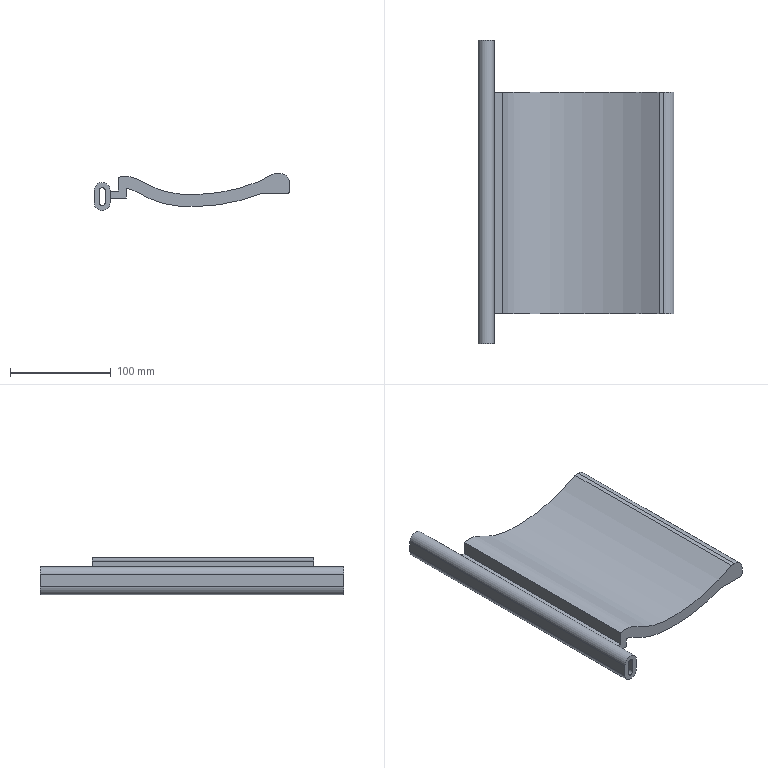Part | SolidWorks | features ExtruThin 1, ICE 1 | 1 solid | 25 faces | box 194.613 x 302 x 37.008 mm | volume 615517 mm3 | plane 15 | cylinder 8 | spline 2 | commonest cylinder face diameters 6 x4 16 x3 20 x1
STEP:
#1=CARTESIAN_POINT('',(3.,2.,-11.497));
#2=VERTEX_POINT('',#1);
#3=CARTESIAN_POINT('',(0.,2.,-14.497));
#4=VERTEX_POINT('',#3);
#5=CARTESIAN_POINT('',(0.,2.,-11.497));
#6=DIRECTION('',(0.,1.,0.));
#7=DIRECTION('',(0.,0.,1.));
#8=AXIS2_PLACEMENT_3D('',#5,#6,#7);
#9=CIRCLE('',#8,3.);
#10=EDGE_CURVE('',#2,#4,#9,.T.);
#11=ORIENTED_EDGE('',*,*,#10,.T.);
#12=CARTESIAN_POINT('',(0.,-300.,-14.497));
#13=VERTEX_POINT('',#12);
#14=CARTESIAN_POINT('',(0.,2.,-14.497));
#15=DIRECTION('',(0.,-1.,0.));
#16=VECTOR('',#15,1000.);
#17=LINE('',#14,#16);
#18=EDGE_CURVE('',#4,#13,#17,.T.);
#19=ORIENTED_EDGE('',*,*,#18,.T.);
#20=CARTESIAN_POINT('',(3.,-300.,-11.497));
#21=VERTEX_POINT('',#20);
#22=CARTESIAN_POINT('',(0.,-300.,-11.497));
#23=DIRECTION('',(0.,1.,0.));
#24=DIRECTION('',(0.,0.,1.));
#25=AXIS2_PLACEMENT_3D('',#22,#23,#24);
#26=CIRCLE('',#25,3.);
#27=EDGE_CURVE('',#21,#13,#26,.T.);
#28=ORIENTED_EDGE('',*,*,#27,.F.);
#29=CARTESIAN_POINT('',(3.,2.,-11.497));
#30=DIRECTION('',(0.,-1.,0.));
#31=VECTOR('',#30,1000.);
#32=LINE('',#29,#31);
#33=EDGE_CURVE('',#2,#21,#32,.T.);
#34=ORIENTED_EDGE('',*,*,#33,.F.);
#35=EDGE_LOOP('',(#11,#19,#28,#34));
#36=FACE_OUTER_BOUND('',#35,.T.);
#37=CARTESIAN_POINT('',(0.,2.,-11.497));
#38=DIRECTION('',(0.,-1.,0.));
#39=DIRECTION('',(0.,0.,-1.));
#40=AXIS2_PLACEMENT_3D('',#37,#38,#39);
#41=CYLINDRICAL_SURFACE('',#40,3.);
#42=ADVANCED_FACE('',(#36),#41,.F.);
#43=CARTESIAN_POINT('',(0.,2.,-19.497));
#44=VERTEX_POINT('',#43);
#45=CARTESIAN_POINT('',(-8.,2.,-11.497));
#46=VERTEX_POINT('',#45);
#47=CARTESIAN_POINT('',(0.,2.,-11.497));
#48=DIRECTION('',(0.,1.,0.));
#49=DIRECTION('',(1.,0.,0.));
#50=AXIS2_PLACEMENT_3D('',#47,#48,#49);
#51=CIRCLE('',#50,8.);
#52=EDGE_CURVE('',#44,#46,#51,.T.);
#53=ORIENTED_EDGE('',*,*,#52,.F.);
#54=CARTESIAN_POINT('',(0.,-300.,-19.497));
#55=VERTEX_POINT('',#54);
#56=CARTESIAN_POINT('',(0.,2.,-19.497));
#57=DIRECTION('',(0.,-1.,0.));
#58=VECTOR('',#57,1000.);
#59=LINE('',#56,#58);
#60=EDGE_CURVE('',#44,#55,#59,.T.);
#61=ORIENTED_EDGE('',*,*,#60,.T.);
#62=CARTESIAN_POINT('',(-8.,-300.,-11.497));
#63=VERTEX_POINT('',#62);
#64=CARTESIAN_POINT('',(0.,-300.,-11.497));
#65=DIRECTION('',(0.,1.,0.));
#66=DIRECTION('',(1.,0.,0.));
#67=AXIS2_PLACEMENT_3D('',#64,#65,#66);
#68=CIRCLE('',#67,8.);
#69=EDGE_CURVE('',#55,#63,#68,.T.);
#70=ORIENTED_EDGE('',*,*,#69,.T.);
#71=CARTESIAN_POINT('',(-8.,2.,-11.497));
#72=DIRECTION('',(0.,-1.,0.));
#73=VECTOR('',#72,1000.);
#74=LINE('',#71,#73);
#75=EDGE_CURVE('',#46,#63,#74,.T.);
#76=ORIENTED_EDGE('',*,*,#75,.F.);
#77=EDGE_LOOP('',(#53,#61,#70,#76));
#78=FACE_OUTER_BOUND('',#77,.T.);
#79=CARTESIAN_POINT('',(0.,2.,-11.497));
#80=DIRECTION('',(0.,-1.,0.));
#81=DIRECTION('',(0.,0.,-1.));
#82=AXIS2_PLACEMENT_3D('',#79,#80,#81);
#83=CYLINDRICAL_SURFACE('',#82,8.);
#84=ADVANCED_FACE('',(#78),#83,.T.);
#85=CARTESIAN_POINT('',(8.,2.,-11.497));
#86=VERTEX_POINT('',#85);
#87=CARTESIAN_POINT('',(0.,2.,-11.497));
#88=DIRECTION('',(0.,1.,0.));
#89=DIRECTION('',(1.,0.,0.));
#90=AXIS2_PLACEMENT_3D('',#87,#88,#89);
#91=CIRCLE('',#90,8.);
#92=EDGE_CURVE('',#86,#44,#91,.T.);
#93=ORIENTED_EDGE('',*,*,#92,.T.);
#94=ORIENTED_EDGE('',*,*,#52,.T.);
#95=CARTESIAN_POINT('',(-8.,2.,0.5032));
#96=VERTEX_POINT('',#95);
#97=CARTESIAN_POINT('',(-8.,2.,-11.497));
#98=DIRECTION('',(0.,0.,1.));
#99=VECTOR('',#98,1000.);
#100=LINE('',#97,#99);
#101=EDGE_CURVE('',#46,#96,#100,.T.);
#102=ORIENTED_EDGE('',*,*,#101,.T.);
#103=CARTESIAN_POINT('',(8.,2.,0.5032));
#104=VERTEX_POINT('',#103);
#105=CARTESIAN_POINT('',(0.,2.,0.5032));
#106=DIRECTION('',(0.,1.,0.));
#107=DIRECTION('',(1.,0.,0.));
#108=AXIS2_PLACEMENT_3D('',#105,#106,#107);
#109=CIRCLE('',#108,8.);
#110=EDGE_CURVE('',#96,#104,#109,.T.);
#111=ORIENTED_EDGE('',*,*,#110,.T.);
#112=CARTESIAN_POINT('',(8.,2.,-11.497));
#113=DIRECTION('',(0.,0.,-1.));
#114=VECTOR('',#113,1000.);
#115=LINE('',#112,#114);
#116=EDGE_CURVE('',#104,#86,#115,.T.);
#117=ORIENTED_EDGE('',*,*,#116,.T.);
#118=EDGE_LOOP('',(#93,#94,#102,#111,#117));
#119=FACE_OUTER_BOUND('',#118,.T.);
#120=CARTESIAN_POINT('',(-3.,2.,-11.497));
#121=VERTEX_POINT('',#120);
#122=CARTESIAN_POINT('',(-3.,2.,0.5032));
#123=VERTEX_POINT('',#122);
#124=CARTESIAN_POINT('',(-3.,2.,-11.497));
#125=DIRECTION('',(0.,0.,1.));
#126=VECTOR('',#125,1000.);
#127=LINE('',#124,#126);
#128=EDGE_CURVE('',#121,#123,#127,.T.);
#129=ORIENTED_EDGE('',*,*,#128,.F.);
#130=CARTESIAN_POINT('',(0.,2.,-11.497));
#131=DIRECTION('',(0.,1.,0.));
#132=DIRECTION('',(0.,0.,1.));
#133=AXIS2_PLACEMENT_3D('',#130,#131,#132);
#134=CIRCLE('',#133,3.);
#135=EDGE_CURVE('',#4,#121,#134,.T.);
#136=ORIENTED_EDGE('',*,*,#135,.F.);
#137=ORIENTED_EDGE('',*,*,#10,.F.);
#138=CARTESIAN_POINT('',(3.,2.,0.5032));
#139=VERTEX_POINT('',#138);
#140=CARTESIAN_POINT('',(3.,2.,-11.497));
#141=DIRECTION('',(0.,0.,-1.));
#142=VECTOR('',#141,1000.);
#143=LINE('',#140,#142);
#144=EDGE_CURVE('',#139,#2,#143,.T.);
#145=ORIENTED_EDGE('',*,*,#144,.F.);
#146=CARTESIAN_POINT('',(0.,2.,0.5032));
#147=DIRECTION('',(0.,1.,0.));
#148=DIRECTION('',(0.,0.,1.));
#149=AXIS2_PLACEMENT_3D('',#146,#147,#148);
#150=CIRCLE('',#149,3.);
#151=EDGE_CURVE('',#123,#139,#150,.T.);
#152=ORIENTED_EDGE('',*,*,#151,.F.);
#153=EDGE_LOOP('',(#129,#136,#137,#145,#152));
#154=FACE_BOUND('',#153,.T.);
#155=CARTESIAN_POINT('',(0.,2.,-11.497));
#156=DIRECTION('',(0.,1.,0.));
#157=DIRECTION('',(0.,0.,1.));
#158=AXIS2_PLACEMENT_3D('',#155,#156,#157);
#159=PLANE('',#158);
#160=ADVANCED_FACE('',(#119,#154),#159,.T.);
#161=ORIENTED_EDGE('',*,*,#60,.F.);
#162=ORIENTED_EDGE('',*,*,#92,.F.);
#163=CARTESIAN_POINT('',(8.,-300.,-11.497));
#164=VERTEX_POINT('',#163);
#165=CARTESIAN_POINT('',(8.,2.,-11.497));
#166=DIRECTION('',(0.,-1.,0.));
#167=VECTOR('',#166,1000.);
#168=LINE('',#165,#167);
#169=EDGE_CURVE('',#86,#164,#168,.T.);
#170=ORIENTED_EDGE('',*,*,#169,.T.);
#171=CARTESIAN_POINT('',(0.,-300.,-11.497));
#172=DIRECTION('',(0.,1.,0.));
#173=DIRECTION('',(1.,0.,0.));
#174=AXIS2_PLACEMENT_3D('',#171,#172,#173);
#175=CIRCLE('',#174,8.);
#176=EDGE_CURVE('',#164,#55,#175,.T.);
#177=ORIENTED_EDGE('',*,*,#176,.T.);
#178=EDGE_LOOP('',(#161,#162,#170,#177));
#179=FACE_OUTER_BOUND('',#178,.T.);
#180=CARTESIAN_POINT('',(0.,2.,-11.497));
#181=DIRECTION('',(0.,-1.,0.));
#182=DIRECTION('',(0.,0.,-1.));
#183=AXIS2_PLACEMENT_3D('',#180,#181,#182);
#184=CYLINDRICAL_SURFACE('',#183,8.);
#185=ADVANCED_FACE('',(#179),#184,.T.);
#186=ORIENTED_EDGE('',*,*,#75,.T.);
#187=CARTESIAN_POINT('',(-8.,-300.,0.5032));
#188=VERTEX_POINT('',#187);
#189=CARTESIAN_POINT('',(-8.,-300.,-11.497));
#190=DIRECTION('',(0.,0.,1.));
#191=VECTOR('',#190,1000.);
#192=LINE('',#189,#191);
#193=EDGE_CURVE('',#63,#188,#192,.T.);
#194=ORIENTED_EDGE('',*,*,#193,.T.);
#195=CARTESIAN_POINT('',(-8.,2.,0.5032));
#196=DIRECTION('',(0.,-1.,0.));
#197=VECTOR('',#196,1000.);
#198=LINE('',#195,#197);
#199=EDGE_CURVE('',#96,#188,#198,.T.);
#200=ORIENTED_EDGE('',*,*,#199,.F.);
#201=ORIENTED_EDGE('',*,*,#101,.F.);
#202=EDGE_LOOP('',(#186,#194,#200,#201));
#203=FACE_OUTER_BOUND('',#202,.T.);
#204=CARTESIAN_POINT('',(-8.,2.,-11.497));
#205=DIRECTION('',(1.,0.,0.));
#206=DIRECTION('',(0.,0.,-1.));
#207=AXIS2_PLACEMENT_3D('',#204,#205,#206);
#208=PLANE('',#207);
#209=ADVANCED_FACE('',(#203),#208,.F.);
#210=ORIENTED_EDGE('',*,*,#199,.T.);
#211=CARTESIAN_POINT('',(8.,-300.,0.5032));
#212=VERTEX_POINT('',#211);
#213=CARTESIAN_POINT('',(0.,-300.,0.5032));
#214=DIRECTION('',(0.,1.,0.));
#215=DIRECTION('',(1.,0.,0.));
#216=AXIS2_PLACEMENT_3D('',#213,#214,#215);
#217=CIRCLE('',#216,8.);
#218=EDGE_CURVE('',#188,#212,#217,.T.);
#219=ORIENTED_EDGE('',*,*,#218,.T.);
#220=CARTESIAN_POINT('',(8.,2.,0.5032));
#221=DIRECTION('',(0.,-1.,0.));
#222=VECTOR('',#221,1000.);
#223=LINE('',#220,#222);
#224=EDGE_CURVE('',#104,#212,#223,.T.);
#225=ORIENTED_EDGE('',*,*,#224,.F.);
#226=ORIENTED_EDGE('',*,*,#110,.F.);
#227=EDGE_LOOP('',(#210,#219,#225,#226));
#228=FACE_OUTER_BOUND('',#227,.T.);
#229=CARTESIAN_POINT('',(0.,2.,0.5032));
#230=DIRECTION('',(0.,-1.,0.));
#231=DIRECTION('',(0.,0.,-1.));
#232=AXIS2_PLACEMENT_3D('',#229,#230,#231);
#233=CYLINDRICAL_SURFACE('',#232,8.);
#234=ADVANCED_FACE('',(#228),#233,.T.);
#235=CARTESIAN_POINT('',(8.,-270.,-7.));
#236=VERTEX_POINT('',#235);
#237=CARTESIAN_POINT('',(8.,-50.,-7.));
#238=VERTEX_POINT('',#237);
#239=CARTESIAN_POINT('',(8.,-270.,-7.));
#240=DIRECTION('',(0.,1.,0.));
#241=VECTOR('',#240,1000.);
#242=LINE('',#239,#241);
#243=EDGE_CURVE('',#236,#238,#242,.T.);
#244=ORIENTED_EDGE('',*,*,#243,.F.);
#245=CARTESIAN_POINT('',(8.,-270.,0.));
#246=VERTEX_POINT('',#245);
#247=CARTESIAN_POINT('',(8.,-270.,0.));
#248=DIRECTION('',(0.,0.,1.));
#249=VECTOR('',#248,1000.);
#250=LINE('',#247,#249);
#251=EDGE_CURVE('',#236,#246,#250,.T.);
#252=ORIENTED_EDGE('',*,*,#251,.T.);
#253=CARTESIAN_POINT('',(8.,-50.,0.));
#254=VERTEX_POINT('',#253);
#255=CARTESIAN_POINT('',(8.,-270.,0.));
#256=DIRECTION('',(0.,1.,0.));
#257=VECTOR('',#256,1000.);
#258=LINE('',#255,#257);
#259=EDGE_CURVE('',#246,#254,#258,.T.);
#260=ORIENTED_EDGE('',*,*,#259,.T.);
#261=CARTESIAN_POINT('',(8.,-50.,0.));
#262=DIRECTION('',(0.,0.,1.));
#263=VECTOR('',#262,1000.);
#264=LINE('',#261,#263);
#265=EDGE_CURVE('',#238,#254,#264,.T.);
#266=ORIENTED_EDGE('',*,*,#265,.F.);
#267=EDGE_LOOP('',(#244,#252,#260,#266));
#268=FACE_BOUND('',#267,.T.);
#269=ORIENTED_EDGE('',*,*,#224,.T.);
#270=CARTESIAN_POINT('',(8.,-300.,-11.497));
#271=DIRECTION('',(0.,0.,-1.));
#272=VECTOR('',#271,1000.);
#273=LINE('',#270,#272);
#274=EDGE_CURVE('',#212,#164,#273,.T.);
#275=ORIENTED_EDGE('',*,*,#274,.T.);
#276=ORIENTED_EDGE('',*,*,#169,.F.);
#277=ORIENTED_EDGE('',*,*,#116,.F.);
#278=EDGE_LOOP('',(#269,#275,#276,#277));
#279=FACE_OUTER_BOUND('',#278,.T.);
#280=CARTESIAN_POINT('',(8.,2.,-11.497));
#281=DIRECTION('',(-1.,0.,0.));
#282=DIRECTION('',(0.,0.,1.));
#283=AXIS2_PLACEMENT_3D('',#280,#281,#282);
#284=PLANE('',#283);
#285=ADVANCED_FACE('',(#268,#279),#284,.F.);
#286=ORIENTED_EDGE('',*,*,#18,.F.);
#287=ORIENTED_EDGE('',*,*,#135,.T.);
#288=CARTESIAN_POINT('',(-3.,-300.,-11.497));
#289=VERTEX_POINT('',#288);
#290=CARTESIAN_POINT('',(-3.,2.,-11.497));
#291=DIRECTION('',(0.,-1.,0.));
#292=VECTOR('',#291,1000.);
#293=LINE('',#290,#292);
#294=EDGE_CURVE('',#121,#289,#293,.T.);
#295=ORIENTED_EDGE('',*,*,#294,.T.);
#296=CARTESIAN_POINT('',(0.,-300.,-11.497));
#297=DIRECTION('',(0.,1.,0.));
#298=DIRECTION('',(0.,0.,1.));
#299=AXIS2_PLACEMENT_3D('',#296,#297,#298);
#300=CIRCLE('',#299,3.);
#301=EDGE_CURVE('',#13,#289,#300,.T.);
#302=ORIENTED_EDGE('',*,*,#301,.F.);
#303=EDGE_LOOP('',(#286,#287,#295,#302));
#304=FACE_OUTER_BOUND('',#303,.T.);
#305=CARTESIAN_POINT('',(0.,2.,-11.497));
#306=DIRECTION('',(0.,-1.,0.));
#307=DIRECTION('',(0.,0.,-1.));
#308=AXIS2_PLACEMENT_3D('',#305,#306,#307);
#309=CYLINDRICAL_SURFACE('',#308,3.);
#310=ADVANCED_FACE('',(#304),#309,.F.);
#311=CARTESIAN_POINT('',(-3.,-300.,0.5032));
#312=VERTEX_POINT('',#311);
#313=CARTESIAN_POINT('',(-3.,2.,0.5032));
#314=DIRECTION('',(0.,-1.,0.));
#315=VECTOR('',#314,1000.);
#316=LINE('',#313,#315);
#317=EDGE_CURVE('',#123,#312,#316,.T.);
#318=ORIENTED_EDGE('',*,*,#317,.T.);
#319=CARTESIAN_POINT('',(-3.,-300.,-11.497));
#320=DIRECTION('',(0.,0.,1.));
#321=VECTOR('',#320,1000.);
#322=LINE('',#319,#321);
#323=EDGE_CURVE('',#289,#312,#322,.T.);
#324=ORIENTED_EDGE('',*,*,#323,.F.);
#325=ORIENTED_EDGE('',*,*,#294,.F.);
#326=ORIENTED_EDGE('',*,*,#128,.T.);
#327=EDGE_LOOP('',(#318,#324,#325,#326));
#328=FACE_OUTER_BOUND('',#327,.T.);
#329=CARTESIAN_POINT('',(-3.,2.,-11.497));
#330=DIRECTION('',(1.,0.,0.));
#331=DIRECTION('',(0.,0.,-1.));
#332=AXIS2_PLACEMENT_3D('',#329,#330,#331);
#333=PLANE('',#332);
#334=ADVANCED_FACE('',(#328),#333,.T.);
#335=CARTESIAN_POINT('',(3.,-300.,0.5032));
#336=VERTEX_POINT('',#335);
#337=CARTESIAN_POINT('',(3.,2.,0.5032));
#338=DIRECTION('',(0.,-1.,0.));
#339=VECTOR('',#338,1000.);
#340=LINE('',#337,#339);
#341=EDGE_CURVE('',#139,#336,#340,.T.);
#342=ORIENTED_EDGE('',*,*,#341,.T.);
#343=CARTESIAN_POINT('',(0.,-300.,0.5032));
#344=DIRECTION('',(0.,1.,0.));
#345=DIRECTION('',(0.,0.,1.));
#346=AXIS2_PLACEMENT_3D('',#343,#344,#345);
#347=CIRCLE('',#346,3.);
#348=EDGE_CURVE('',#312,#336,#347,.T.);
#349=ORIENTED_EDGE('',*,*,#348,.F.);
#350=ORIENTED_EDGE('',*,*,#317,.F.);
#351=ORIENTED_EDGE('',*,*,#151,.T.);
#352=EDGE_LOOP('',(#342,#349,#350,#351));
#353=FACE_OUTER_BOUND('',#352,.T.);
#354=CARTESIAN_POINT('',(0.,2.,0.5032));
#355=DIRECTION('',(0.,-1.,0.));
#356=DIRECTION('',(0.,0.,-1.));
#357=AXIS2_PLACEMENT_3D('',#354,#355,#356);
#358=CYLINDRICAL_SURFACE('',#357,3.);
#359=ADVANCED_FACE('',(#353),#358,.F.);
#360=ORIENTED_EDGE('',*,*,#33,.T.);
#361=CARTESIAN_POINT('',(3.,-300.,-11.497));
#362=DIRECTION('',(0.,0.,-1.));
#363=VECTOR('',#362,1000.);
#364=LINE('',#361,#363);
#365=EDGE_CURVE('',#336,#21,#364,.T.);
#366=ORIENTED_EDGE('',*,*,#365,.F.);
#367=ORIENTED_EDGE('',*,*,#341,.F.);
#368=ORIENTED_EDGE('',*,*,#144,.T.);
#369=EDGE_LOOP('',(#360,#366,#367,#368));
#370=FACE_OUTER_BOUND('',#369,.T.);
#371=CARTESIAN_POINT('',(3.,2.,-11.497));
#372=DIRECTION('',(-1.,0.,0.));
#373=DIRECTION('',(0.,0.,1.));
#374=AXIS2_PLACEMENT_3D('',#371,#372,#373);
#375=PLANE('',#374);
#376=ADVANCED_FACE('',(#370),#375,.T.);
#377=ORIENTED_EDGE('',*,*,#365,.T.);
#378=ORIENTED_EDGE('',*,*,#27,.T.);
#379=ORIENTED_EDGE('',*,*,#301,.T.);
#380=ORIENTED_EDGE('',*,*,#323,.T.);
#381=ORIENTED_EDGE('',*,*,#348,.T.);
#382=EDGE_LOOP('',(#377,#378,#379,#380,#381));
#383=FACE_BOUND('',#382,.T.);
#384=ORIENTED_EDGE('',*,*,#176,.F.);
#385=ORIENTED_EDGE('',*,*,#274,.F.);
#386=ORIENTED_EDGE('',*,*,#218,.F.);
#387=ORIENTED_EDGE('',*,*,#193,.F.);
#388=ORIENTED_EDGE('',*,*,#69,.F.);
#389=EDGE_LOOP('',(#384,#385,#386,#387,#388));
#390=FACE_OUTER_BOUND('',#389,.T.);
#391=CARTESIAN_POINT('',(0.,-300.,-11.497));
#392=DIRECTION('',(0.,1.,0.));
#393=DIRECTION('',(0.,0.,1.));
#394=AXIS2_PLACEMENT_3D('',#391,#392,#393);
#395=PLANE('',#394);
#396=ADVANCED_FACE('',(#383,#390),#395,.F.);
#397=CARTESIAN_POINT('',(24.,-50.,-7.));
#398=VERTEX_POINT('',#397);
#399=CARTESIAN_POINT('',(8.,-50.,-7.));
#400=DIRECTION('',(-1.,0.,0.));
#401=VECTOR('',#400,1000.);
#402=LINE('',#399,#401);
#403=EDGE_CURVE('',#398,#238,#402,.T.);
#404=ORIENTED_EDGE('',*,*,#403,.F.);
#405=CARTESIAN_POINT('',(24.,-270.,-7.));
#406=VERTEX_POINT('',#405);
#407=CARTESIAN_POINT('',(24.,-270.,-7.));
#408=DIRECTION('',(0.,1.,0.));
#409=VECTOR('',#408,1000.);
#410=LINE('',#407,#409);
#411=EDGE_CURVE('',#406,#398,#410,.T.);
#412=ORIENTED_EDGE('',*,*,#411,.F.);
#413=CARTESIAN_POINT('',(8.,-270.,-7.));
#414=DIRECTION('',(-1.,0.,0.));
#415=VECTOR('',#414,1000.);
#416=LINE('',#413,#415);
#417=EDGE_CURVE('',#406,#236,#416,.T.);
#418=ORIENTED_EDGE('',*,*,#417,.T.);
#419=ORIENTED_EDGE('',*,*,#243,.T.);
#420=EDGE_LOOP('',(#404,#412,#418,#419));
#421=FACE_OUTER_BOUND('',#420,.T.);
#422=CARTESIAN_POINT('',(8.,-270.,-7.));
#423=DIRECTION('',(0.,0.,-1.));
#424=DIRECTION('',(-1.,0.,0.));
#425=AXIS2_PLACEMENT_3D('',#422,#423,#424);
#426=PLANE('',#425);
#427=ADVANCED_FACE('',(#421),#426,.T.);
#428=CARTESIAN_POINT('',(24.,-50.,2.515));
#429=VERTEX_POINT('',#428);
#430=CARTESIAN_POINT('',(24.,-50.,-7.));
#431=DIRECTION('',(0.,0.,-1.));
#432=VECTOR('',#431,1000.);
#433=LINE('',#430,#432);
#434=EDGE_CURVE('',#429,#398,#433,.T.);
#435=ORIENTED_EDGE('',*,*,#434,.F.);
#436=CARTESIAN_POINT('',(24.,-270.,2.515));
#437=VERTEX_POINT('',#436);
#438=CARTESIAN_POINT('',(24.,-270.,2.515));
#439=DIRECTION('',(0.,1.,0.));
#440=VECTOR('',#439,1000.);
#441=LINE('',#438,#440);
#442=EDGE_CURVE('',#437,#429,#441,.T.);
#443=ORIENTED_EDGE('',*,*,#442,.F.);
#444=CARTESIAN_POINT('',(24.,-270.,-7.));
#445=DIRECTION('',(0.,0.,-1.));
#446=VECTOR('',#445,1000.);
#447=LINE('',#444,#446);
#448=EDGE_CURVE('',#437,#406,#447,.T.);
#449=ORIENTED_EDGE('',*,*,#448,.T.);
#450=ORIENTED_EDGE('',*,*,#411,.T.);
#451=EDGE_LOOP('',(#435,#443,#449,#450));
#452=FACE_OUTER_BOUND('',#451,.T.);
#453=CARTESIAN_POINT('',(24.,-270.,-7.));
#454=DIRECTION('',(1.,0.,0.));
#455=DIRECTION('',(0.,0.,-1.));
#456=AXIS2_PLACEMENT_3D('',#453,#454,#455);
#457=PLANE('',#456);
#458=ADVANCED_FACE('',(#452),#457,.T.);
#459=CARTESIAN_POINT('',(158.,-50.,-2.488));
#460=VERTEX_POINT('',#459);
#461=CARTESIAN_POINT('',(158.,-50.,-2.488));
#462=CARTESIAN_POINT('',(157.156,-50.,-2.831));
#463=CARTESIAN_POINT('',(150.375,-50.,-5.52));
#464=CARTESIAN_POINT('',(136.567,-50.,-9.992));
#465=CARTESIAN_POINT('',(119.729,-50.,-13.363));
#466=CARTESIAN_POINT('',(105.362,-50.,-14.956));
#467=CARTESIAN_POINT('',(96.312,-50.,-15.443));
#468=CARTESIAN_POINT('',(89.056,-50.,-15.54));
#469=CARTESIAN_POINT('',(81.665,-50.,-15.421));
#470=CARTESIAN_POINT('',(74.121,-50.,-14.875));
#471=CARTESIAN_POINT('',(66.495,-50.,-13.703));
#472=CARTESIAN_POINT('',(60.758,-50.,-12.456));
#473=CARTESIAN_POINT('',(55.983,-50.,-11.063));
#474=CARTESIAN_POINT('',(52.193,-50.,-9.711));
#475=CARTESIAN_POINT('',(49.349,-50.,-8.563));
#476=CARTESIAN_POINT('',(46.601,-50.,-7.315));
#477=CARTESIAN_POINT('',(43.16,-50.,-5.617));
#478=CARTESIAN_POINT('',(39.186,-50.,-3.501));
#479=CARTESIAN_POINT('',(34.88,-50.,-1.214));
#480=CARTESIAN_POINT('',(31.01,-50.,0.6263));
#481=CARTESIAN_POINT('',(27.601,-50.,1.883));
#482=CARTESIAN_POINT('',(25.51,-50.,2.342));
#483=CARTESIAN_POINT('',(24.35,-50.,2.482));
#484=CARTESIAN_POINT('',(24.113,-50.,2.505));
#485=CARTESIAN_POINT('',(24.,-50.,2.515));
#486=B_SPLINE_CURVE_WITH_KNOTS('',3,(#461,#462,#463,#464,#465,#466,#467,#468,#469,#470,#471,#472,#473,#474,#475,#476,#477,#478,#479,#480,#481,#482,#483,#484,#485),.UNSPECIFIED.,.F.,.F.,(4,1,1,1,1,1,1,1,1,1,1,1,1,1,1,1,1,1,1,1,1,1,4),(0.1247,0.1404,0.25,0.375,0.4375,0.5,0.5312,0.5625,0.625,0.6562,0.6875,0.7188,0.7344,0.75,0.7656,0.7812,0.8125,0.8438,0.875,0.9062,0.9375,0.9417,0.9457),.UNSPECIFIED.);
#487=EDGE_CURVE('',#460,#429,#486,.T.);
#488=ORIENTED_EDGE('',*,*,#487,.F.);
#489=CARTESIAN_POINT('',(158.,-270.,-2.488));
#490=VERTEX_POINT('',#489);
#491=CARTESIAN_POINT('',(158.,-270.,-2.488));
#492=DIRECTION('',(0.,1.,0.));
#493=VECTOR('',#492,1000.);
#494=LINE('',#491,#493);
#495=EDGE_CURVE('',#490,#460,#494,.T.);
#496=ORIENTED_EDGE('',*,*,#495,.F.);
#497=CARTESIAN_POINT('',(158.,-270.,-2.488));
#498=CARTESIAN_POINT('',(157.156,-270.,-2.831));
#499=CARTESIAN_POINT('',(150.375,-270.,-5.52));
#500=CARTESIAN_POINT('',(136.567,-270.,-9.992));
#501=CARTESIAN_POINT('',(119.729,-270.,-13.363));
#502=CARTESIAN_POINT('',(105.362,-270.,-14.956));
#503=CARTESIAN_POINT('',(96.312,-270.,-15.443));
#504=CARTESIAN_POINT('',(89.056,-270.,-15.54));
#505=CARTESIAN_POINT('',(81.665,-270.,-15.421));
#506=CARTESIAN_POINT('',(74.121,-270.,-14.875));
#507=CARTESIAN_POINT('',(66.495,-270.,-13.703));
#508=CARTESIAN_POINT('',(60.758,-270.,-12.456));
#509=CARTESIAN_POINT('',(55.983,-270.,-11.063));
#510=CARTESIAN_POINT('',(52.193,-270.,-9.711));
#511=CARTESIAN_POINT('',(49.349,-270.,-8.563));
#512=CARTESIAN_POINT('',(46.601,-270.,-7.315));
#513=CARTESIAN_POINT('',(43.16,-270.,-5.617));
#514=CARTESIAN_POINT('',(39.186,-270.,-3.501));
#515=CARTESIAN_POINT('',(34.88,-270.,-1.214));
#516=CARTESIAN_POINT('',(31.01,-270.,0.6263));
#517=CARTESIAN_POINT('',(27.601,-270.,1.883));
#518=CARTESIAN_POINT('',(25.51,-270.,2.342));
#519=CARTESIAN_POINT('',(24.35,-270.,2.482));
#520=CARTESIAN_POINT('',(24.113,-270.,2.505));
#521=CARTESIAN_POINT('',(24.,-270.,2.515));
#522=B_SPLINE_CURVE_WITH_KNOTS('',3,(#497,#498,#499,#500,#501,#502,#503,#504,#505,#506,#507,#508,#509,#510,#511,#512,#513,#514,#515,#516,#517,#518,#519,#520,#521),.UNSPECIFIED.,.F.,.F.,(4,1,1,1,1,1,1,1,1,1,1,1,1,1,1,1,1,1,1,1,1,1,4),(0.1247,0.1404,0.25,0.375,0.4375,0.5,0.5312,0.5625,0.625,0.6562,0.6875,0.7188,0.7344,0.75,0.7656,0.7812,0.8125,0.8438,0.875,0.9062,0.9375,0.9417,0.9457),.UNSPECIFIED.);
#523=EDGE_CURVE('',#490,#437,#522,.T.);
#524=ORIENTED_EDGE('',*,*,#523,.T.);
#525=ORIENTED_EDGE('',*,*,#442,.T.);
#526=EDGE_LOOP('',(#488,#496,#524,#525));
#527=FACE_OUTER_BOUND('',#526,.T.);
#528=CARTESIAN_POINT('',(158.,-270.,-2.488));
#529=CARTESIAN_POINT('',(158.,-50.,-2.488));
#530=CARTESIAN_POINT('',(157.156,-270.,-2.831));
#531=CARTESIAN_POINT('',(157.156,-50.,-2.831));
#532=CARTESIAN_POINT('',(150.375,-270.,-5.52));
#533=CARTESIAN_POINT('',(150.375,-50.,-5.52));
#534=CARTESIAN_POINT('',(136.567,-270.,-9.992));
#535=CARTESIAN_POINT('',(136.567,-50.,-9.992));
#536=CARTESIAN_POINT('',(119.729,-270.,-13.363));
#537=CARTESIAN_POINT('',(119.729,-50.,-13.363));
#538=CARTESIAN_POINT('',(105.362,-270.,-14.956));
#539=CARTESIAN_POINT('',(105.362,-50.,-14.956));
#540=CARTESIAN_POINT('',(96.312,-270.,-15.443));
#541=CARTESIAN_POINT('',(96.312,-50.,-15.443));
#542=CARTESIAN_POINT('',(89.056,-270.,-15.54));
#543=CARTESIAN_POINT('',(89.056,-50.,-15.54));
#544=CARTESIAN_POINT('',(81.665,-270.,-15.421));
#545=CARTESIAN_POINT('',(81.665,-50.,-15.421));
#546=CARTESIAN_POINT('',(74.121,-270.,-14.875));
#547=CARTESIAN_POINT('',(74.121,-50.,-14.875));
#548=CARTESIAN_POINT('',(66.495,-270.,-13.703));
#549=CARTESIAN_POINT('',(66.495,-50.,-13.703));
#550=CARTESIAN_POINT('',(60.758,-270.,-12.456));
#551=CARTESIAN_POINT('',(60.758,-50.,-12.456));
#552=CARTESIAN_POINT('',(55.983,-270.,-11.063));
#553=CARTESIAN_POINT('',(55.983,-50.,-11.063));
#554=CARTESIAN_POINT('',(52.193,-270.,-9.711));
#555=CARTESIAN_POINT('',(52.193,-50.,-9.711));
#556=CARTESIAN_POINT('',(49.349,-270.,-8.563));
#557=CARTESIAN_POINT('',(49.349,-50.,-8.563));
#558=CARTESIAN_POINT('',(46.601,-270.,-7.315));
#559=CARTESIAN_POINT('',(46.601,-50.,-7.315));
#560=CARTESIAN_POINT('',(43.16,-270.,-5.617));
#561=CARTESIAN_POINT('',(43.16,-50.,-5.617));
#562=CARTESIAN_POINT('',(39.186,-270.,-3.501));
#563=CARTESIAN_POINT('',(39.186,-50.,-3.501));
#564=CARTESIAN_POINT('',(34.88,-270.,-1.214));
#565=CARTESIAN_POINT('',(34.88,-50.,-1.214));
#566=CARTESIAN_POINT('',(31.01,-270.,0.6263));
#567=CARTESIAN_POINT('',(31.01,-50.,0.6263));
#568=CARTESIAN_POINT('',(27.601,-270.,1.883));
#569=CARTESIAN_POINT('',(27.601,-50.,1.883));
#570=CARTESIAN_POINT('',(25.51,-270.,2.342));
#571=CARTESIAN_POINT('',(25.51,-50.,2.342));
#572=CARTESIAN_POINT('',(24.35,-270.,2.482));
#573=CARTESIAN_POINT('',(24.35,-50.,2.482));
#574=CARTESIAN_POINT('',(24.113,-270.,2.505));
#575=CARTESIAN_POINT('',(24.113,-50.,2.505));
#576=CARTESIAN_POINT('',(24.,-270.,2.515));
#577=CARTESIAN_POINT('',(24.,-50.,2.515));
#578=B_SPLINE_SURFACE_WITH_KNOTS('',3,1,((#528,#529),(#530,#531),(#532,#533),(#534,#535),(#536,#537),(#538,#539),(#540,#541),(#542,#543),(#544,#545),(#546,#547),(#548,#549),(#550,#551),(#552,#553),(#554,#555),(#556,#557),(#558,#559),(#560,#561),(#562,#563),(#564,#565),(#566,#567),(#568,#569),(#570,#571),(#572,#573),(#574,#575),(#576,#577)),.UNSPECIFIED.,.F.,.F.,.F.,(4,1,1,1,1,1,1,1,1,1,1,1,1,1,1,1,1,1,1,1,1,1,4),(2,2),(0.1247,0.1404,0.25,0.375,0.4375,0.5,0.5312,0.5625,0.625,0.6562,0.6875,0.7188,0.7344,0.75,0.7656,0.7812,0.8125,0.8438,0.875,0.9062,0.9375,0.9417,0.9457),(0.,1.),.UNSPECIFIED.);
#579=ADVANCED_FACE('',(#527),#578,.T.);
#580=CARTESIAN_POINT('',(183.613,-50.,-2.488));
#581=VERTEX_POINT('',#580);
#582=CARTESIAN_POINT('',(158.,-50.,-2.488));
#583=DIRECTION('',(-1.,0.,0.));
#584=VECTOR('',#583,1000.);
#585=LINE('',#582,#584);
#586=EDGE_CURVE('',#581,#460,#585,.T.);
#587=ORIENTED_EDGE('',*,*,#586,.F.);
#588=CARTESIAN_POINT('',(183.613,-270.,-2.488));
#589=VERTEX_POINT('',#588);
#590=CARTESIAN_POINT('',(183.613,-270.,-2.488));
#591=DIRECTION('',(0.,1.,0.));
#592=VECTOR('',#591,1000.);
#593=LINE('',#590,#592);
#594=EDGE_CURVE('',#589,#581,#593,.T.);
#595=ORIENTED_EDGE('',*,*,#594,.F.);
#596=CARTESIAN_POINT('',(158.,-270.,-2.488));
#597=DIRECTION('',(-1.,0.,0.));
#598=VECTOR('',#597,1000.);
#599=LINE('',#596,#598);
#600=EDGE_CURVE('',#589,#490,#599,.T.);
#601=ORIENTED_EDGE('',*,*,#600,.T.);
#602=ORIENTED_EDGE('',*,*,#495,.T.);
#603=EDGE_LOOP('',(#587,#595,#601,#602));
#604=FACE_OUTER_BOUND('',#603,.T.);
#605=CARTESIAN_POINT('',(158.,-270.,-2.488));
#606=DIRECTION('',(0.,0.,-1.));
#607=DIRECTION('',(-1.,0.,0.));
#608=AXIS2_PLACEMENT_3D('',#605,#606,#607);
#609=PLANE('',#608);
#610=ADVANCED_FACE('',(#604),#609,.T.);
#611=CARTESIAN_POINT('',(186.613,-50.,0.5115));
#612=VERTEX_POINT('',#611);
#613=CARTESIAN_POINT('',(183.613,-50.,0.5115));
#614=DIRECTION('',(0.,1.,0.));
#615=DIRECTION('',(0.,0.,1.));
#616=AXIS2_PLACEMENT_3D('',#613,#614,#615);
#617=CIRCLE('',#616,3.);
#618=EDGE_CURVE('',#612,#581,#617,.T.);
#619=ORIENTED_EDGE('',*,*,#618,.F.);
#620=CARTESIAN_POINT('',(186.613,-270.,0.5115));
#621=VERTEX_POINT('',#620);
#622=CARTESIAN_POINT('',(186.613,-270.,0.5115));
#623=DIRECTION('',(0.,1.,0.));
#624=VECTOR('',#623,1000.);
#625=LINE('',#622,#624);
#626=EDGE_CURVE('',#621,#612,#625,.T.);
#627=ORIENTED_EDGE('',*,*,#626,.F.);
#628=CARTESIAN_POINT('',(183.613,-270.,0.5115));
#629=DIRECTION('',(0.,1.,0.));
#630=DIRECTION('',(0.,0.,1.));
#631=AXIS2_PLACEMENT_3D('',#628,#629,#630);
#632=CIRCLE('',#631,3.);
#633=EDGE_CURVE('',#621,#589,#632,.T.);
#634=ORIENTED_EDGE('',*,*,#633,.T.);
#635=ORIENTED_EDGE('',*,*,#594,.T.);
#636=EDGE_LOOP('',(#619,#627,#634,#635));
#637=FACE_OUTER_BOUND('',#636,.T.);
#638=CARTESIAN_POINT('',(183.613,-270.,0.5115));
#639=DIRECTION('',(0.,1.,0.));
#640=DIRECTION('',(0.,0.,1.));
#641=AXIS2_PLACEMENT_3D('',#638,#639,#640);
#642=CYLINDRICAL_SURFACE('',#641,3.);
#643=ADVANCED_FACE('',(#637),#642,.T.);
#644=CARTESIAN_POINT('',(186.613,-50.,7.512));
#645=VERTEX_POINT('',#644);
#646=CARTESIAN_POINT('',(186.613,-50.,7.512));
#647=DIRECTION('',(0.,0.,-1.));
#648=VECTOR('',#647,1000.);
#649=LINE('',#646,#648);
#650=EDGE_CURVE('',#645,#612,#649,.T.);
#651=ORIENTED_EDGE('',*,*,#650,.F.);
#652=CARTESIAN_POINT('',(186.613,-270.,7.512));
#653=VERTEX_POINT('',#652);
#654=CARTESIAN_POINT('',(186.613,-270.,7.512));
#655=DIRECTION('',(0.,1.,0.));
#656=VECTOR('',#655,1000.);
#657=LINE('',#654,#656);
#658=EDGE_CURVE('',#653,#645,#657,.T.);
#659=ORIENTED_EDGE('',*,*,#658,.F.);
#660=CARTESIAN_POINT('',(186.613,-270.,7.512));
#661=DIRECTION('',(0.,0.,-1.));
#662=VECTOR('',#661,1000.);
#663=LINE('',#660,#662);
#664=EDGE_CURVE('',#653,#621,#663,.T.);
#665=ORIENTED_EDGE('',*,*,#664,.T.);
#666=ORIENTED_EDGE('',*,*,#626,.T.);
#667=EDGE_LOOP('',(#651,#659,#665,#666));
#668=FACE_OUTER_BOUND('',#667,.T.);
#669=CARTESIAN_POINT('',(186.613,-270.,7.512));
#670=DIRECTION('',(1.,0.,0.));
#671=DIRECTION('',(0.,0.,-1.));
#672=AXIS2_PLACEMENT_3D('',#669,#670,#671);
#673=PLANE('',#672);
#674=ADVANCED_FACE('',(#668),#673,.T.);
#675=CARTESIAN_POINT('',(176.613,-50.,17.512));
#676=VERTEX_POINT('',#675);
#677=CARTESIAN_POINT('',(176.613,-50.,7.512));
#678=DIRECTION('',(0.,1.,0.));
#679=DIRECTION('',(0.,0.,1.));
#680=AXIS2_PLACEMENT_3D('',#677,#678,#679);
#681=CIRCLE('',#680,10.);
#682=EDGE_CURVE('',#676,#645,#681,.T.);
#683=ORIENTED_EDGE('',*,*,#682,.F.);
#684=CARTESIAN_POINT('',(176.613,-270.,17.512));
#685=VERTEX_POINT('',#684);
#686=CARTESIAN_POINT('',(176.613,-270.,17.512));
#687=DIRECTION('',(0.,1.,0.));
#688=VECTOR('',#687,1000.);
#689=LINE('',#686,#688);
#690=EDGE_CURVE('',#685,#676,#689,.T.);
#691=ORIENTED_EDGE('',*,*,#690,.F.);
#692=CARTESIAN_POINT('',(176.613,-270.,7.512));
#693=DIRECTION('',(0.,1.,0.));
#694=DIRECTION('',(0.,0.,1.));
#695=AXIS2_PLACEMENT_3D('',#692,#693,#694);
#696=CIRCLE('',#695,10.);
#697=EDGE_CURVE('',#685,#653,#696,.T.);
#698=ORIENTED_EDGE('',*,*,#697,.T.);
#699=ORIENTED_EDGE('',*,*,#658,.T.);
#700=EDGE_LOOP('',(#683,#691,#698,#699));
#701=FACE_OUTER_BOUND('',#700,.T.);
#702=CARTESIAN_POINT('',(176.613,-270.,7.512));
#703=DIRECTION('',(0.,1.,0.));
#704=DIRECTION('',(0.,0.,1.));
#705=AXIS2_PLACEMENT_3D('',#702,#703,#704);
#706=CYLINDRICAL_SURFACE('',#705,10.);
#707=ADVANCED_FACE('',(#701),#706,.T.);
#708=CARTESIAN_POINT('',(171.849,-50.,17.512));
#709=VERTEX_POINT('',#708);
#710=CARTESIAN_POINT('',(171.849,-50.,17.512));
#711=DIRECTION('',(1.,0.,0.));
#712=VECTOR('',#711,1000.);
#713=LINE('',#710,#712);
#714=EDGE_CURVE('',#709,#676,#713,.T.);
#715=ORIENTED_EDGE('',*,*,#714,.F.);
#716=CARTESIAN_POINT('',(171.849,-270.,17.512));
#717=VERTEX_POINT('',#716);
#718=CARTESIAN_POINT('',(171.849,-270.,17.512));
#719=DIRECTION('',(0.,1.,0.));
#720=VECTOR('',#719,1000.);
#721=LINE('',#718,#720);
#722=EDGE_CURVE('',#717,#709,#721,.T.);
#723=ORIENTED_EDGE('',*,*,#722,.F.);
#724=CARTESIAN_POINT('',(171.849,-270.,17.512));
#725=DIRECTION('',(1.,0.,0.));
#726=VECTOR('',#725,1000.);
#727=LINE('',#724,#726);
#728=EDGE_CURVE('',#717,#685,#727,.T.);
#729=ORIENTED_EDGE('',*,*,#728,.T.);
#730=ORIENTED_EDGE('',*,*,#690,.T.);
#731=EDGE_LOOP('',(#715,#723,#729,#730));
#732=FACE_OUTER_BOUND('',#731,.T.);
#733=CARTESIAN_POINT('',(171.849,-270.,17.512));
#734=DIRECTION('',(0.,0.,1.));
#735=DIRECTION('',(1.,0.,0.));
#736=AXIS2_PLACEMENT_3D('',#733,#734,#735);
#737=PLANE('',#736);
#738=ADVANCED_FACE('',(#732),#737,.T.);
#739=CARTESIAN_POINT('',(16.,-50.,13.621));
#740=VERTEX_POINT('',#739);
#741=CARTESIAN_POINT('',(16.,-50.,13.621));
#742=CARTESIAN_POINT('',(30.5,-50.,17.645));
#743=CARTESIAN_POINT('',(51.936,-50.,-1.311));
#744=CARTESIAN_POINT('',(107.31,-50.,-6.157));
#745=CARTESIAN_POINT('',(147.097,-50.,3.485));
#746=CARTESIAN_POINT('',(171.849,-50.,17.512));
#747=B_SPLINE_CURVE_WITH_KNOTS('',3,(#741,#742,#743,#744,#745,#746),.UNSPECIFIED.,.F.,.F.,(4,1,1,4),(0.,0.2503,0.4832,1.),.UNSPECIFIED.);
#748=EDGE_CURVE('',#740,#709,#747,.T.);
#749=ORIENTED_EDGE('',*,*,#748,.F.);
#750=CARTESIAN_POINT('',(16.,-270.,13.621));
#751=VERTEX_POINT('',#750);
#752=CARTESIAN_POINT('',(16.,-270.,13.621));
#753=DIRECTION('',(0.,1.,0.));
#754=VECTOR('',#753,1000.);
#755=LINE('',#752,#754);
#756=EDGE_CURVE('',#751,#740,#755,.T.);
#757=ORIENTED_EDGE('',*,*,#756,.F.);
#758=CARTESIAN_POINT('',(16.,-270.,13.621));
#759=CARTESIAN_POINT('',(30.5,-270.,17.645));
#760=CARTESIAN_POINT('',(51.936,-270.,-1.311));
#761=CARTESIAN_POINT('',(107.31,-270.,-6.157));
#762=CARTESIAN_POINT('',(147.097,-270.,3.485));
#763=CARTESIAN_POINT('',(171.849,-270.,17.512));
#764=B_SPLINE_CURVE_WITH_KNOTS('',3,(#758,#759,#760,#761,#762,#763),.UNSPECIFIED.,.F.,.F.,(4,1,1,4),(0.,0.2503,0.4832,1.),.UNSPECIFIED.);
#765=EDGE_CURVE('',#751,#717,#764,.T.);
#766=ORIENTED_EDGE('',*,*,#765,.T.);
#767=ORIENTED_EDGE('',*,*,#722,.T.);
#768=EDGE_LOOP('',(#749,#757,#766,#767));
#769=FACE_OUTER_BOUND('',#768,.T.);
#770=CARTESIAN_POINT('',(16.,-270.,13.621));
#771=CARTESIAN_POINT('',(16.,-50.,13.621));
#772=CARTESIAN_POINT('',(30.5,-270.,17.645));
#773=CARTESIAN_POINT('',(30.5,-50.,17.645));
#774=CARTESIAN_POINT('',(51.936,-270.,-1.311));
#775=CARTESIAN_POINT('',(51.936,-50.,-1.311));
#776=CARTESIAN_POINT('',(107.31,-270.,-6.157));
#777=CARTESIAN_POINT('',(107.31,-50.,-6.157));
#778=CARTESIAN_POINT('',(147.097,-270.,3.485));
#779=CARTESIAN_POINT('',(147.097,-50.,3.485));
#780=CARTESIAN_POINT('',(171.849,-270.,17.512));
#781=CARTESIAN_POINT('',(171.849,-50.,17.512));
#782=B_SPLINE_SURFACE_WITH_KNOTS('',3,1,((#770,#771),(#772,#773),(#774,#775),(#776,#777),(#778,#779),(#780,#781)),.UNSPECIFIED.,.F.,.F.,.F.,(4,1,1,4),(2,2),(0.,0.2503,0.4832,1.),(0.,1.),.UNSPECIFIED.);
#783=ADVANCED_FACE('',(#769),#782,.T.);
#784=CARTESIAN_POINT('',(16.,-50.,0.));
#785=VERTEX_POINT('',#784);
#786=CARTESIAN_POINT('',(16.,-50.,0.));
#787=DIRECTION('',(0.,0.,1.));
#788=VECTOR('',#787,1000.);
#789=LINE('',#786,#788);
#790=EDGE_CURVE('',#785,#740,#789,.T.);
#791=ORIENTED_EDGE('',*,*,#790,.F.);
#792=CARTESIAN_POINT('',(16.,-270.,0.));
#793=VERTEX_POINT('',#792);
#794=CARTESIAN_POINT('',(16.,-270.,0.));
#795=DIRECTION('',(0.,1.,0.));
#796=VECTOR('',#795,1000.);
#797=LINE('',#794,#796);
#798=EDGE_CURVE('',#793,#785,#797,.T.);
#799=ORIENTED_EDGE('',*,*,#798,.F.);
#800=CARTESIAN_POINT('',(16.,-270.,0.));
#801=DIRECTION('',(0.,0.,1.));
#802=VECTOR('',#801,1000.);
#803=LINE('',#800,#802);
#804=EDGE_CURVE('',#793,#751,#803,.T.);
#805=ORIENTED_EDGE('',*,*,#804,.T.);
#806=ORIENTED_EDGE('',*,*,#756,.T.);
#807=EDGE_LOOP('',(#791,#799,#805,#806));
#808=FACE_OUTER_BOUND('',#807,.T.);
#809=CARTESIAN_POINT('',(16.,-270.,0.));
#810=DIRECTION('',(-1.,0.,0.));
#811=DIRECTION('',(0.,0.,1.));
#812=AXIS2_PLACEMENT_3D('',#809,#810,#811);
#813=PLANE('',#812);
#814=ADVANCED_FACE('',(#808),#813,.T.);
#815=CARTESIAN_POINT('',(8.,-50.,0.));
#816=DIRECTION('',(1.,0.,0.));
#817=VECTOR('',#816,1000.);
#818=LINE('',#815,#817);
#819=EDGE_CURVE('',#254,#785,#818,.T.);
#820=ORIENTED_EDGE('',*,*,#819,.F.);
#821=ORIENTED_EDGE('',*,*,#259,.F.);
#822=CARTESIAN_POINT('',(8.,-270.,0.));
#823=DIRECTION('',(1.,0.,0.));
#824=VECTOR('',#823,1000.);
#825=LINE('',#822,#824);
#826=EDGE_CURVE('',#246,#793,#825,.T.);
#827=ORIENTED_EDGE('',*,*,#826,.T.);
#828=ORIENTED_EDGE('',*,*,#798,.T.);
#829=EDGE_LOOP('',(#820,#821,#827,#828));
#830=FACE_OUTER_BOUND('',#829,.T.);
#831=CARTESIAN_POINT('',(8.,-270.,0.));
#832=DIRECTION('',(0.,0.,1.));
#833=DIRECTION('',(1.,0.,0.));
#834=AXIS2_PLACEMENT_3D('',#831,#832,#833);
#835=PLANE('',#834);
#836=ADVANCED_FACE('',(#830),#835,.T.);
#837=ORIENTED_EDGE('',*,*,#251,.F.);
#838=ORIENTED_EDGE('',*,*,#417,.F.);
#839=ORIENTED_EDGE('',*,*,#448,.F.);
#840=ORIENTED_EDGE('',*,*,#523,.F.);
#841=ORIENTED_EDGE('',*,*,#600,.F.);
#842=ORIENTED_EDGE('',*,*,#633,.F.);
#843=ORIENTED_EDGE('',*,*,#664,.F.);
#844=ORIENTED_EDGE('',*,*,#697,.F.);
#845=ORIENTED_EDGE('',*,*,#728,.F.);
#846=ORIENTED_EDGE('',*,*,#765,.F.);
#847=ORIENTED_EDGE('',*,*,#804,.F.);
#848=ORIENTED_EDGE('',*,*,#826,.F.);
#849=EDGE_LOOP('',(#837,#838,#839,#840,#841,#842,#843,#844,#845,#846,#847,#848));
#850=FACE_OUTER_BOUND('',#849,.T.);
#851=CARTESIAN_POINT('',(94.496,-270.,-15.443));
#852=DIRECTION('',(0.,-1.,0.));
#853=DIRECTION('',(0.,0.,-1.));
#854=AXIS2_PLACEMENT_3D('',#851,#852,#853);
#855=PLANE('',#854);
#856=ADVANCED_FACE('',(#850),#855,.T.);
#857=ORIENTED_EDGE('',*,*,#265,.T.);
#858=ORIENTED_EDGE('',*,*,#819,.T.);
#859=ORIENTED_EDGE('',*,*,#790,.T.);
#860=ORIENTED_EDGE('',*,*,#748,.T.);
#861=ORIENTED_EDGE('',*,*,#714,.T.);
#862=ORIENTED_EDGE('',*,*,#682,.T.);
#863=ORIENTED_EDGE('',*,*,#650,.T.);
#864=ORIENTED_EDGE('',*,*,#618,.T.);
#865=ORIENTED_EDGE('',*,*,#586,.T.);
#866=ORIENTED_EDGE('',*,*,#487,.T.);
#867=ORIENTED_EDGE('',*,*,#434,.T.);
#868=ORIENTED_EDGE('',*,*,#403,.T.);
#869=EDGE_LOOP('',(#857,#858,#859,#860,#861,#862,#863,#864,#865,#866,#867,#868));
#870=FACE_OUTER_BOUND('',#869,.T.);
#871=CARTESIAN_POINT('',(94.496,-50.,-15.443));
#872=DIRECTION('',(0.,-1.,0.));
#873=DIRECTION('',(0.,0.,-1.));
#874=AXIS2_PLACEMENT_3D('',#871,#872,#873);
#875=PLANE('',#874);
#876=ADVANCED_FACE('',(#870),#875,.F.);
#877=CLOSED_SHELL('',(#42,#84,#160,#185,#209,#234,#285,#310,#334,#359,#376,#396,#427,#458,#579,#610,#643,#674,#707,#738,#783,#814,#836,#856,#876));
#878=MANIFOLD_SOLID_BREP('',#877);
#879=CARTESIAN_POINT('',(0.,0.,0.));
#880=DIRECTION('',(0.,0.,1.));
#881=DIRECTION('',(1.,0.,0.));
#882=AXIS2_PLACEMENT_3D('',#879,#880,#881);
#883=(LENGTH_UNIT()NAMED_UNIT(*)SI_UNIT(.MILLI.,.METRE.));
#884=UNCERTAINTY_MEASURE_WITH_UNIT(LENGTH_MEASURE(0.00001),#883,'','');
#885=(NAMED_UNIT(*)PLANE_ANGLE_UNIT()SI_UNIT($,.RADIAN.));
#886=(NAMED_UNIT(*)SI_UNIT($,.STERADIAN.)SOLID_ANGLE_UNIT());
#887=(GEOMETRIC_REPRESENTATION_CONTEXT(3)GLOBAL_UNCERTAINTY_ASSIGNED_CONTEXT((#884))GLOBAL_UNIT_ASSIGNED_CONTEXT((#883,#885,#886))REPRESENTATION_CONTEXT('',''));
#888=ADVANCED_BREP_SHAPE_REPRESENTATION('',(#878,#882),#887);